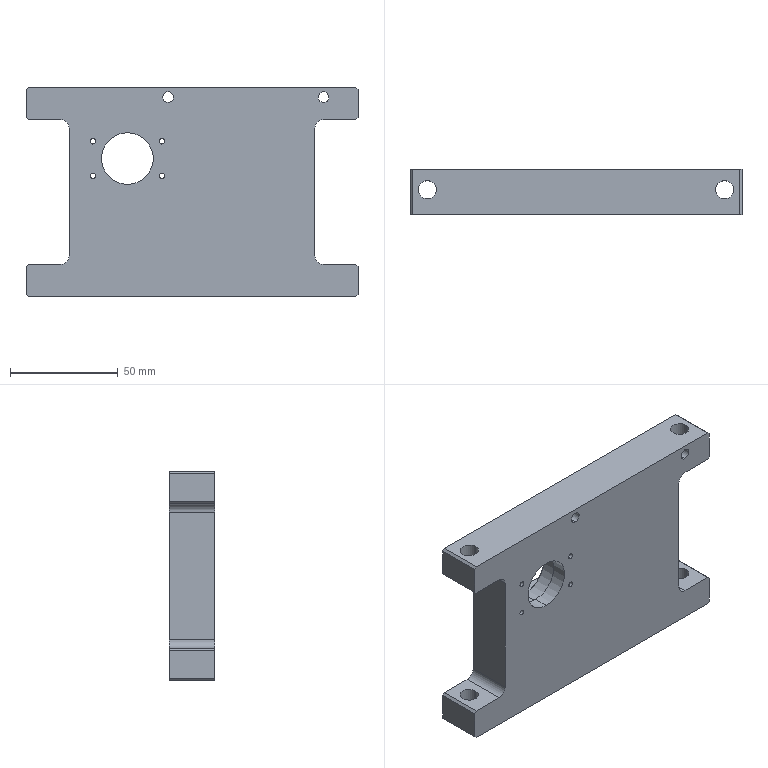Part | STEP file | Front Guide Channel Support Plate Right | 1 solid | 77 faces | box 154 x 21 x 97 mm | volume 228293 mm3 | cylinder 40 | plane 31 | cone 6 | commonest cylinder face diameters 2.5 x8 8.5 x8 4 x4 5 x4 8 x4 16 x4